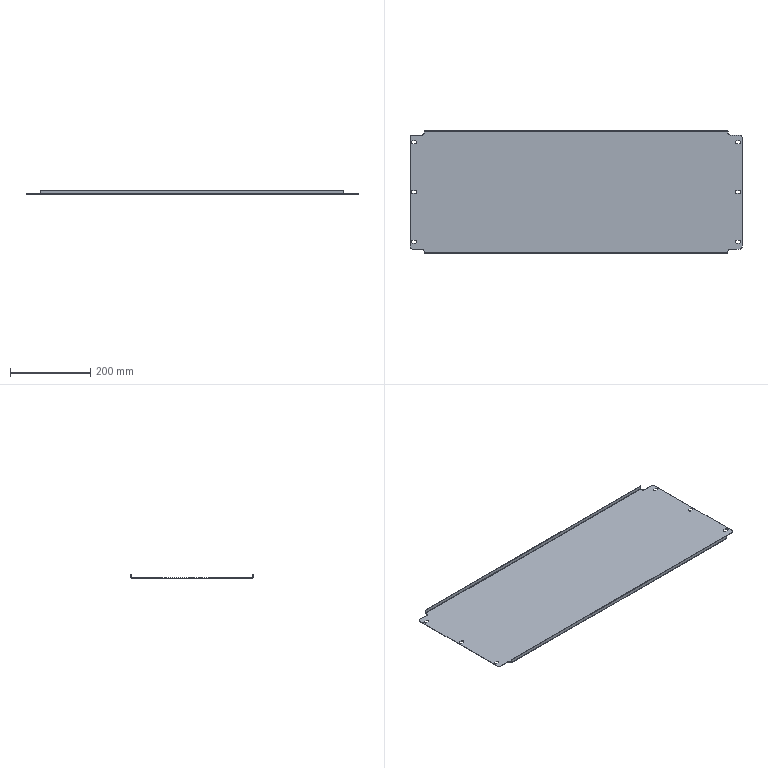Part | SolidWorks | features ICE 3, Cut 1, EdgeFlange 1, Fillet 1, FlatPattern 1, SMBaseFlange 1, SheetMetal 1 | 1 solid | 68 faces | box 830 x 305 x 10 mm | volume 264295 mm3 | plane 38 | cylinder 30 | commonest cylinder face diameters 7 x18 10 x8 1 x2 3 x2